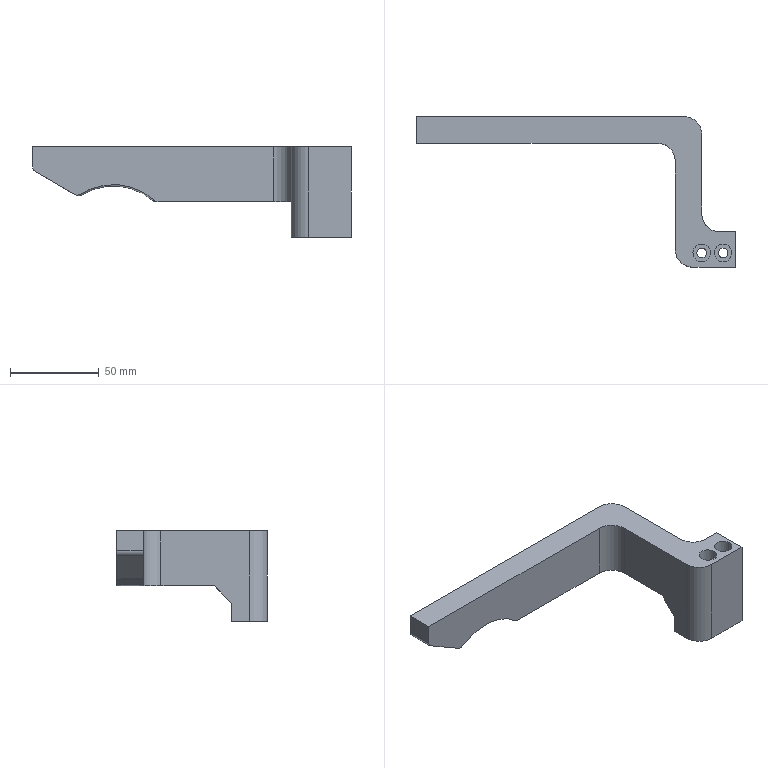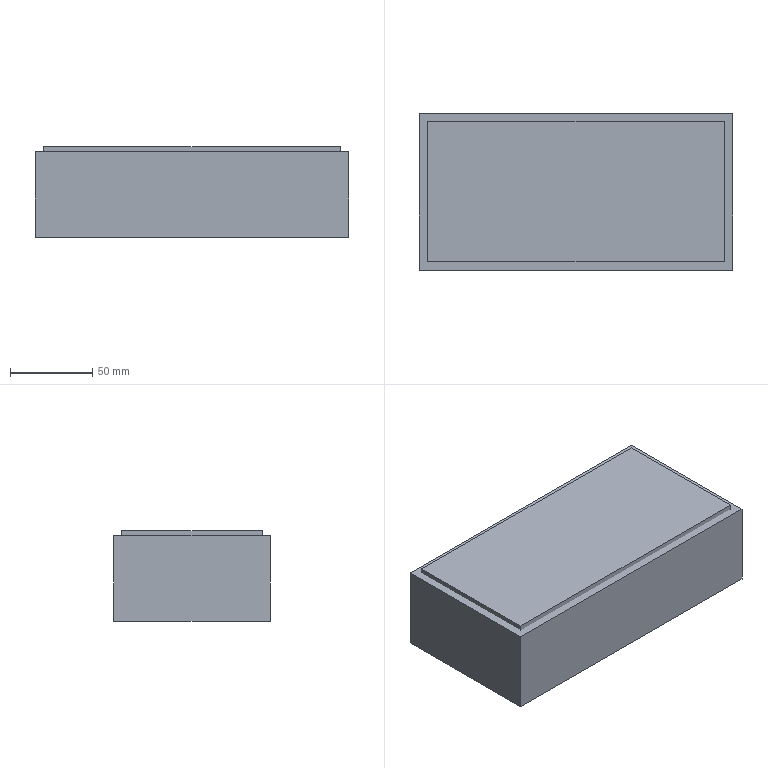CAM job | NX | 3-axis milling, drilling | part box 180 x 85 x 51 mm | stock box 190 x 95 x 55 mm
Tools:
number,name,description,diameter,corner_radius,flute_length,length,flutes
1,D63,Milling Tool-5 Parameters,63.0,0.0,50.0,75.0,2
12,D12C,Milling Tool-5 Parameters,12.0,0.0,50.0,75.0,2
10,D10,Milling Tool-5 Parameters,10.0,0.0,50.0,75.0,2
11,D12JING,Milling Tool-5 Parameters,12.0,0.0,50.0,75.0,2
5,D4R0.5,Milling Tool-5 Parameters,4.0,0.5,50.0,75.0,2
8,R4,Milling Tool-5 Parameters,8.0,4.0,50.0,75.0,2
7,D6A45,Milling Tool-5 Parameters,6.0,0.0,50.0,75.0,2
15,5.5ZT,Drilling Tool,5.5,0.0,35.0,50.0,2
6,D6,Milling Tool-5 Parameters,6.0,0.0,50.0,75.0,2
Operations:
program,operation,operation_type,tool,method,geometry_group,spindle_rpm,surface_speed,feed_per_tooth,feed_cut,feed_plunge,cut_length_mm,path_length_mm,cut_time_min,machine_time_min
1,FLOOR_WALL,VolumeBased25DMillingOperation,D63,METHOD,A,6500.0,1286.0,0.1154,1500.0,100.0,840.797,894.797,0.5605,0.5659
1,ADAPTIVE_MILLING,CavityMilling,D12C,METHOD,A,9500.0,358.0,0.1579,3000.0,1000.0,45896.718,49662.445,15.329,15.706
1,ADAPTIVE_MILLING_COPY,CavityMilling,D12C,METHOD,A,9500.0,358.0,0.1579,3000.0,1000.0,46647.314,59768.62,15.629,16.941
1,FLOOR_WALL_COPY,VolumeBased25DMillingOperation,D63,METHOD,A,6500.0,1286.0,0.1154,1500.0,100.0,5061.063,11315.129,3.374,3.999
1,ZLEVEL_PROFILE,ZLevelMilling,D12C,METHOD,A,9500.0,358.0,0.1316,2500.0,1000.0,957.473,1021.763,0.3874,0.3939
1,ZLEVEL_PROFILE_COPY,ZLevelMilling,D12C,METHOD,A,9500.0,358.0,0.1316,2500.0,1000.0,688.573,772.968,0.2803,0.2887
1,ZLEVEL_PROFILE_COPY_COPY_COPY,ZLevelMilling,D12C,METHOD,A,9500.0,358.0,0.1316,2500.0,1000.0,1172.983,1302.498,0.4781,0.491
1,ZLEVEL_PROFILE_COPY_COPY,ZLevelMilling,D12C,METHOD,A,9500.0,358.0,0.1316,2500.0,1000.0,1078.178,1755.819,0.4592,0.527
1,ZLEVEL_PROFILE_COPY_COPY_COPY_1,ZLevelMilling,D10,METHOD,A,9500.0,358.0,0.1316,2500.0,1000.0,2393.604,2483.804,1.064,1.073
1,ZLEVEL_PROFILE_COPY_COPY_COPY_1_COPY,ZLevelMilling,D12JING,METHOD,A,9500.0,358.0,0.0632,1200.0,1000.0,134.336,224.736,0.1144,0.1235
1,ZLEVEL_PROFILE_COPY_COPY_COPY_1_COPY_COPY,ZLevelMilling,D12JING,METHOD,A,9500.0,358.0,0.0632,1200.0,1000.0,42.633,122.433,0.0362,0.0442
1,ZLEVEL_PROFILE_COPY_COPY_COPY_1_COPY_COPY_COPY,ZLevelMilling,D12JING,METHOD,A,9500.0,358.0,0.0632,1200.0,1000.0,1119.524,1282.098,0.9344,0.9507
1,ZLEVEL_PROFILE_COPY_COPY_COPY_COPY,ZLevelMilling,D4R0.5,METHOD,A,9500.0,119.0,0.1316,2500.0,1000.0,2541.487,2625.846,1.019,1.028
1,FIXED_CONTOUR,SurfaceContour,R4,METHOD,A,9500.0,119.0,0.1316,2500.0,100.0,14035.706,14149.993,5.614,5.626
1,PLANAR_MILL,PlanarMilling,D6A45,METHOD,A,9500.0,179.0,0.0658,1250.0,100.0,172.437,232.437,0.1379,0.1439
1,PLANAR_MILL_COPY,PlanarMilling,D6A45,METHOD,A,9500.0,179.0,0.0658,1250.0,100.0,255.935,474.608,0.2047,0.2266
2,FLOOR_WALL_COPY_1,VolumeBased25DMillingOperation,D63,METHOD,B,6500.0,1286.0,0.1154,1500.0,100.0,3203.188,4175.427,2.135,2.233
2,DRILLING,Operation,D6A45,METHOD,B,5000.0,94.0,0.025,250.0,0.0,8.0,91.369,0.032,0.0403
2,DRILLING_COPY,Operation,5.5ZT,METHOD,B,2000.0,34.0,0.0625,250.0,0.0,83.905,243.179,0.3356,0.3515
2,HOLE_MILLING,CylinderMilling,D6,METHOD,B,9500.0,179.0,0.0447,850.0,100.0,1926.977,2109.577,2.267,2.285
2,PLANAR_MILL_COPY_1,PlanarMilling,D6A45,METHOD,B,9500.0,179.0,0.0658,1250.0,100.0,582.292,895.678,0.4658,0.4972